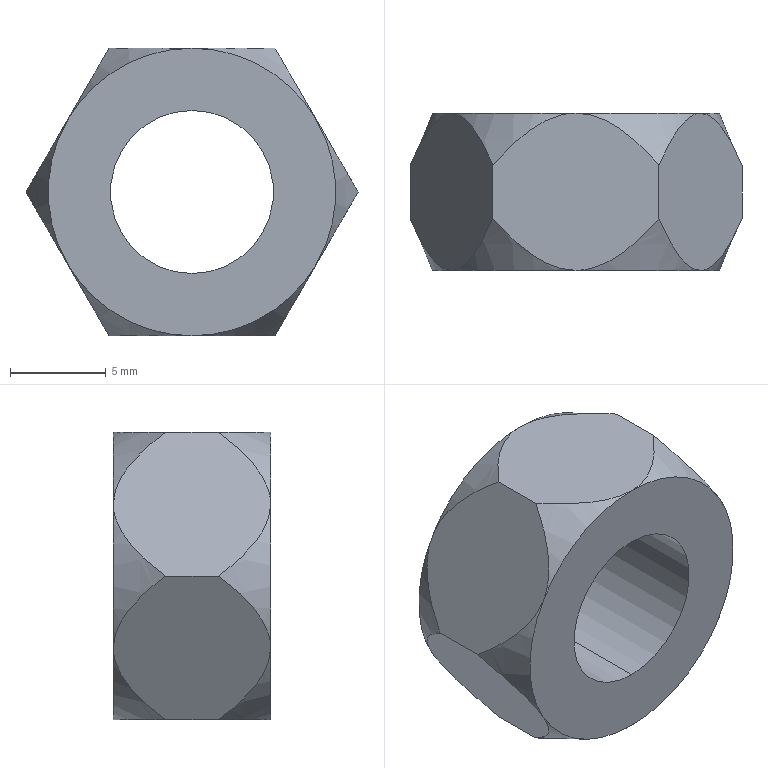Part | SolidWorks | features ICE 2, Extrusion 1, HoleWzd 1 | 1 solid | 24 faces | box 17.321 x 8.2 x 15 mm | volume 1094 mm3 | cone 14 | plane 8 | cylinder 2 | commonest cylinder face diameters 8.5 x2
STEP:
#1=CARTESIAN_POINT('',(0.,7.425,-4.25));
#2=VERTEX_POINT('',#1);
#3=CARTESIAN_POINT('',(0.,7.425,4.25));
#4=VERTEX_POINT('',#3);
#5=CARTESIAN_POINT('',(0.,7.425,0.));
#6=DIRECTION('',(0.,1.,0.));
#7=DIRECTION('',(0.,0.,1.));
#8=AXIS2_PLACEMENT_3D('',#5,#6,#7);
#9=CIRCLE('',#8,4.25);
#10=EDGE_CURVE('',#2,#4,#9,.T.);
#11=ORIENTED_EDGE('',*,*,#10,.F.);
#12=CARTESIAN_POINT('',(0.,8.2,-5.025));
#13=VERTEX_POINT('',#12);
#14=CARTESIAN_POINT('',(0.,8.2,-5.025));
#15=DIRECTION('',(0.,0.7071,-0.7071));
#16=VECTOR('',#15,1000.);
#17=LINE('',#14,#16);
#18=EDGE_CURVE('',#2,#13,#17,.T.);
#19=ORIENTED_EDGE('',*,*,#18,.T.);
#20=CARTESIAN_POINT('',(0.,8.2,5.025));
#21=VERTEX_POINT('',#20);
#22=CARTESIAN_POINT('',(0.,8.2,0.));
#23=DIRECTION('',(0.,1.,0.));
#24=DIRECTION('',(0.,0.,1.));
#25=AXIS2_PLACEMENT_3D('',#22,#23,#24);
#26=CIRCLE('',#25,5.025);
#27=EDGE_CURVE('',#13,#21,#26,.T.);
#28=ORIENTED_EDGE('',*,*,#27,.T.);
#29=CARTESIAN_POINT('',(0.,8.2,5.025));
#30=DIRECTION('',(0.,0.7071,0.7071));
#31=VECTOR('',#30,1000.);
#32=LINE('',#29,#31);
#33=EDGE_CURVE('',#4,#21,#32,.T.);
#34=ORIENTED_EDGE('',*,*,#33,.F.);
#35=EDGE_LOOP('',(#11,#19,#28,#34));
#36=FACE_OUTER_BOUND('',#35,.T.);
#37=CARTESIAN_POINT('',(0.,8.2,0.));
#38=DIRECTION('',(0.,1.,0.));
#39=DIRECTION('',(0.,0.,1.));
#40=AXIS2_PLACEMENT_3D('',#37,#38,#39);
#41=CONICAL_SURFACE('',#40,5.025,0.7854);
#42=ADVANCED_FACE('',(#36),#41,.F.);
#43=CARTESIAN_POINT('',(0.,0.,-4.25));
#44=VERTEX_POINT('',#43);
#45=CARTESIAN_POINT('',(0.,0.,4.25));
#46=VERTEX_POINT('',#45);
#47=CARTESIAN_POINT('',(0.,0.,0.));
#48=DIRECTION('',(0.,1.,0.));
#49=DIRECTION('',(0.,0.,1.));
#50=AXIS2_PLACEMENT_3D('',#47,#48,#49);
#51=CIRCLE('',#50,4.25);
#52=EDGE_CURVE('',#44,#46,#51,.T.);
#53=ORIENTED_EDGE('',*,*,#52,.F.);
#54=CARTESIAN_POINT('',(0.,8.2,-4.25));
#55=DIRECTION('',(0.,1.,0.));
#56=VECTOR('',#55,1000.);
#57=LINE('',#54,#56);
#58=EDGE_CURVE('',#44,#2,#57,.T.);
#59=ORIENTED_EDGE('',*,*,#58,.T.);
#60=ORIENTED_EDGE('',*,*,#10,.T.);
#61=CARTESIAN_POINT('',(0.,8.2,4.25));
#62=DIRECTION('',(0.,1.,0.));
#63=VECTOR('',#62,1000.);
#64=LINE('',#61,#63);
#65=EDGE_CURVE('',#46,#4,#64,.T.);
#66=ORIENTED_EDGE('',*,*,#65,.F.);
#67=EDGE_LOOP('',(#53,#59,#60,#66));
#68=FACE_OUTER_BOUND('',#67,.T.);
#69=CARTESIAN_POINT('',(0.,8.2,0.));
#70=DIRECTION('',(0.,1.,0.));
#71=DIRECTION('',(0.,0.,1.));
#72=AXIS2_PLACEMENT_3D('',#69,#70,#71);
#73=CYLINDRICAL_SURFACE('',#72,4.25);
#74=ADVANCED_FACE('',(#68),#73,.F.);
#75=CARTESIAN_POINT('',(4.33,2.733,-7.5));
#76=VERTEX_POINT('',#75);
#77=CARTESIAN_POINT('',(6.495,0.,-3.75));
#78=VERTEX_POINT('',#77);
#79=CARTESIAN_POINT('',(4.33,2.733,-7.5));
#80=CARTESIAN_POINT('',(4.473,2.397,-7.253));
#81=CARTESIAN_POINT('',(4.621,2.073,-6.997));
#82=CARTESIAN_POINT('',(4.933,1.46,-6.456));
#83=CARTESIAN_POINT('',(5.097,1.172,-6.172));
#84=CARTESIAN_POINT('',(5.452,0.6535,-5.557));
#85=CARTESIAN_POINT('',(5.645,0.4234,-5.223));
#86=CARTESIAN_POINT('',(5.952,0.1778,-4.69));
#87=CARTESIAN_POINT('',(6.06,0.1115,-4.504));
#88=CARTESIAN_POINT('',(6.276,0.02274,-4.129));
#89=CARTESIAN_POINT('',(6.385,0.,-3.94));
#90=CARTESIAN_POINT('',(6.495,0.,-3.75));
#91=B_SPLINE_CURVE_WITH_KNOTS('',3,(#79,#80,#81,#82,#83,#84,#85,#86,#87,#88,#89,#90),.UNSPECIFIED.,.F.,.F.,(4,2,2,2,2,4),(0.000000354,0.001312,0.002623,0.003934,0.00459,0.005245),.UNSPECIFIED.);
#92=EDGE_CURVE('',#76,#78,#91,.T.);
#93=ORIENTED_EDGE('',*,*,#92,.F.);
#94=CARTESIAN_POINT('',(4.33,5.467,-7.5));
#95=VERTEX_POINT('',#94);
#96=CARTESIAN_POINT('',(4.33,8.2,-7.5));
#97=DIRECTION('',(0.,-1.,0.));
#98=VECTOR('',#97,1000.);
#99=LINE('',#96,#98);
#100=EDGE_CURVE('',#95,#76,#99,.T.);
#101=ORIENTED_EDGE('',*,*,#100,.F.);
#102=CARTESIAN_POINT('',(6.495,8.2,-3.75));
#103=VERTEX_POINT('',#102);
#104=CARTESIAN_POINT('',(6.495,8.2,-3.75));
#105=CARTESIAN_POINT('',(6.386,8.2,-3.939));
#106=CARTESIAN_POINT('',(6.275,8.177,-4.132));
#107=CARTESIAN_POINT('',(6.059,8.088,-4.506));
#108=CARTESIAN_POINT('',(5.954,8.023,-4.688));
#109=CARTESIAN_POINT('',(5.749,7.86,-5.043));
#110=CARTESIAN_POINT('',(5.649,7.761,-5.216));
#111=CARTESIAN_POINT('',(5.459,7.543,-5.545));
#112=CARTESIAN_POINT('',(5.367,7.422,-5.704));
#113=CARTESIAN_POINT('',(5.102,7.036,-6.164));
#114=CARTESIAN_POINT('',(4.935,6.744,-6.452));
#115=CARTESIAN_POINT('',(4.621,6.128,-6.996));
#116=CARTESIAN_POINT('',(4.473,5.803,-7.253));
#117=CARTESIAN_POINT('',(4.33,5.467,-7.5));
#118=B_SPLINE_CURVE_WITH_KNOTS('',3,(#104,#105,#106,#107,#108,#109,#110,#111,#112,#113,#114,#115,#116,#117),.UNSPECIFIED.,.F.,.F.,(4,2,2,2,2,2,4),(0.005245,0.005897,0.00655,0.007202,0.007854,0.009159,0.01046),.UNSPECIFIED.);
#119=EDGE_CURVE('',#103,#95,#118,.T.);
#120=ORIENTED_EDGE('',*,*,#119,.F.);
#121=CARTESIAN_POINT('',(8.66,5.467,0.));
#122=VERTEX_POINT('',#121);
#123=CARTESIAN_POINT('',(8.66,5.467,0.));
#124=CARTESIAN_POINT('',(8.518,5.803,-0.247));
#125=CARTESIAN_POINT('',(8.37,6.127,-0.5033));
#126=CARTESIAN_POINT('',(8.058,6.74,-1.044));
#127=CARTESIAN_POINT('',(7.893,7.028,-1.328));
#128=CARTESIAN_POINT('',(7.538,7.546,-1.943));
#129=CARTESIAN_POINT('',(7.345,7.777,-2.277));
#130=CARTESIAN_POINT('',(7.038,8.022,-2.81));
#131=CARTESIAN_POINT('',(6.931,8.088,-2.996));
#132=CARTESIAN_POINT('',(6.714,8.177,-3.371));
#133=CARTESIAN_POINT('',(6.605,8.2,-3.56));
#134=CARTESIAN_POINT('',(6.495,8.2,-3.75));
#135=B_SPLINE_CURVE_WITH_KNOTS('',3,(#123,#124,#125,#126,#127,#128,#129,#130,#131,#132,#133,#134),.UNSPECIFIED.,.F.,.F.,(4,2,2,2,2,4),(0.000000354,0.001312,0.002623,0.003934,0.00459,0.005245),.UNSPECIFIED.);
#136=EDGE_CURVE('',#122,#103,#135,.T.);
#137=ORIENTED_EDGE('',*,*,#136,.F.);
#138=CARTESIAN_POINT('',(8.66,2.733,0.));
#139=VERTEX_POINT('',#138);
#140=CARTESIAN_POINT('',(8.66,8.2,0.));
#141=DIRECTION('',(0.,-1.,0.));
#142=VECTOR('',#141,1000.);
#143=LINE('',#140,#142);
#144=EDGE_CURVE('',#122,#139,#143,.T.);
#145=ORIENTED_EDGE('',*,*,#144,.T.);
#146=CARTESIAN_POINT('',(6.495,0.,-3.75));
#147=CARTESIAN_POINT('',(6.604,0.,-3.561));
#148=CARTESIAN_POINT('',(6.716,0.02322,-3.368));
#149=CARTESIAN_POINT('',(6.932,0.1121,-2.994));
#150=CARTESIAN_POINT('',(7.037,0.1769,-2.812));
#151=CARTESIAN_POINT('',(7.242,0.3403,-2.457));
#152=CARTESIAN_POINT('',(7.341,0.4391,-2.284));
#153=CARTESIAN_POINT('',(7.532,0.6574,-1.955));
#154=CARTESIAN_POINT('',(7.623,0.7777,-1.796));
#155=CARTESIAN_POINT('',(7.889,1.164,-1.336));
#156=CARTESIAN_POINT('',(8.055,1.456,-1.048));
#157=CARTESIAN_POINT('',(8.369,2.072,-0.504));
#158=CARTESIAN_POINT('',(8.518,2.397,-0.2471));
#159=CARTESIAN_POINT('',(8.66,2.733,0.));
#160=B_SPLINE_CURVE_WITH_KNOTS('',3,(#146,#147,#148,#149,#150,#151,#152,#153,#154,#155,#156,#157,#158,#159),.UNSPECIFIED.,.F.,.F.,(4,2,2,2,2,2,4),(0.005245,0.005897,0.00655,0.007202,0.007854,0.009159,0.01046),.UNSPECIFIED.);
#161=EDGE_CURVE('',#78,#139,#160,.T.);
#162=ORIENTED_EDGE('',*,*,#161,.F.);
#163=EDGE_LOOP('',(#93,#101,#120,#137,#145,#162));
#164=FACE_OUTER_BOUND('',#163,.T.);
#165=CARTESIAN_POINT('',(8.66,8.2,0.));
#166=DIRECTION('',(-0.866,0.,0.5));
#167=DIRECTION('',(0.5,0.,0.866));
#168=AXIS2_PLACEMENT_3D('',#165,#166,#167);
#169=PLANE('',#168);
#170=ADVANCED_FACE('',(#164),#169,.F.);
#171=CARTESIAN_POINT('',(-4.33,2.733,-7.5));
#172=VERTEX_POINT('',#171);
#173=CARTESIAN_POINT('',(0.,0.,-7.5));
#174=VERTEX_POINT('',#173);
#175=CARTESIAN_POINT('',(-4.33,2.733,-7.5));
#176=CARTESIAN_POINT('',(-4.046,2.398,-7.5));
#177=CARTESIAN_POINT('',(-3.75,2.074,-7.5));
#178=CARTESIAN_POINT('',(-3.125,1.461,-7.5));
#179=CARTESIAN_POINT('',(-2.797,1.172,-7.5));
#180=CARTESIAN_POINT('',(-2.261,0.781,-7.5));
#181=CARTESIAN_POINT('',(-2.075,0.6583,-7.5));
#182=CARTESIAN_POINT('',(-1.692,0.4386,-7.5));
#183=CARTESIAN_POINT('',(-1.494,0.3408,-7.5));
#184=CARTESIAN_POINT('',(-1.082,0.1766,-7.5));
#185=CARTESIAN_POINT('',(-0.8685,0.1109,-7.5));
#186=CARTESIAN_POINT('',(-0.4388,0.02303,-7.5));
#187=CARTESIAN_POINT('',(-0.221,0.,-7.5));
#188=CARTESIAN_POINT('',(0.,0.,-7.5));
#189=B_SPLINE_CURVE_WITH_KNOTS('',3,(#175,#176,#177,#178,#179,#180,#181,#182,#183,#184,#185,#186,#187,#188),.UNSPECIFIED.,.F.,.F.,(4,2,2,2,2,2,4),(0.02003,0.02134,0.02266,0.02332,0.02398,0.02464,0.02529),.UNSPECIFIED.);
#190=EDGE_CURVE('',#172,#174,#189,.T.);
#191=ORIENTED_EDGE('',*,*,#190,.F.);
#192=CARTESIAN_POINT('',(-4.33,5.467,-7.5));
#193=VERTEX_POINT('',#192);
#194=CARTESIAN_POINT('',(-4.33,8.2,-7.5));
#195=DIRECTION('',(0.,-1.,0.));
#196=VECTOR('',#195,1000.);
#197=LINE('',#194,#196);
#198=EDGE_CURVE('',#193,#172,#197,.T.);
#199=ORIENTED_EDGE('',*,*,#198,.F.);
#200=CARTESIAN_POINT('',(0.,8.2,-7.5));
#201=VERTEX_POINT('',#200);
#202=CARTESIAN_POINT('',(0.,8.2,-7.5));
#203=CARTESIAN_POINT('',(-0.2209,8.2,-7.5));
#204=CARTESIAN_POINT('',(-0.4444,8.176,-7.5));
#205=CARTESIAN_POINT('',(-0.8758,8.087,-7.5));
#206=CARTESIAN_POINT('',(-1.087,8.022,-7.5));
#207=CARTESIAN_POINT('',(-1.707,7.774,-7.5));
#208=CARTESIAN_POINT('',(-2.084,7.548,-7.5));
#209=CARTESIAN_POINT('',(-2.618,7.159,-7.5));
#210=CARTESIAN_POINT('',(-2.791,7.02,-7.5));
#211=CARTESIAN_POINT('',(-3.125,6.731,-7.5));
#212=CARTESIAN_POINT('',(-3.286,6.581,-7.5));
#213=CARTESIAN_POINT('',(-3.754,6.121,-7.5));
#214=CARTESIAN_POINT('',(-4.048,5.799,-7.5));
#215=CARTESIAN_POINT('',(-4.33,5.467,-7.5));
#216=B_SPLINE_CURVE_WITH_KNOTS('',3,(#202,#203,#204,#205,#206,#207,#208,#209,#210,#211,#212,#213,#214,#215),.UNSPECIFIED.,.F.,.F.,(4,2,2,2,2,2,4),(0.02529,0.02595,0.02661,0.02793,0.02858,0.02924,0.03056),.UNSPECIFIED.);
#217=EDGE_CURVE('',#201,#193,#216,.T.);
#218=ORIENTED_EDGE('',*,*,#217,.F.);
#219=CARTESIAN_POINT('',(4.33,5.467,-7.5));
#220=CARTESIAN_POINT('',(4.046,5.802,-7.5));
#221=CARTESIAN_POINT('',(3.75,6.126,-7.5));
#222=CARTESIAN_POINT('',(3.125,6.739,-7.5));
#223=CARTESIAN_POINT('',(2.797,7.028,-7.5));
#224=CARTESIAN_POINT('',(2.261,7.419,-7.5));
#225=CARTESIAN_POINT('',(2.075,7.542,-7.5));
#226=CARTESIAN_POINT('',(1.692,7.761,-7.5));
#227=CARTESIAN_POINT('',(1.494,7.859,-7.5));
#228=CARTESIAN_POINT('',(1.082,8.023,-7.5));
#229=CARTESIAN_POINT('',(0.8685,8.089,-7.5));
#230=CARTESIAN_POINT('',(0.4388,8.177,-7.5));
#231=CARTESIAN_POINT('',(0.221,8.2,-7.5));
#232=CARTESIAN_POINT('',(0.,8.2,-7.5));
#233=B_SPLINE_CURVE_WITH_KNOTS('',3,(#219,#220,#221,#222,#223,#224,#225,#226,#227,#228,#229,#230,#231,#232),.UNSPECIFIED.,.F.,.F.,(4,2,2,2,2,2,4),(0.02003,0.02134,0.02266,0.02332,0.02398,0.02464,0.02529),.UNSPECIFIED.);
#234=EDGE_CURVE('',#95,#201,#233,.T.);
#235=ORIENTED_EDGE('',*,*,#234,.F.);
#236=ORIENTED_EDGE('',*,*,#100,.T.);
#237=CARTESIAN_POINT('',(0.,0.,-7.5));
#238=CARTESIAN_POINT('',(0.2209,0.,-7.5));
#239=CARTESIAN_POINT('',(0.4444,0.02374,-7.5));
#240=CARTESIAN_POINT('',(0.8758,0.1129,-7.5));
#241=CARTESIAN_POINT('',(1.087,0.178,-7.5));
#242=CARTESIAN_POINT('',(1.707,0.4264,-7.5));
#243=CARTESIAN_POINT('',(2.084,0.6522,-7.5));
#244=CARTESIAN_POINT('',(2.618,1.041,-7.5));
#245=CARTESIAN_POINT('',(2.791,1.18,-7.5));
#246=CARTESIAN_POINT('',(3.125,1.469,-7.5));
#247=CARTESIAN_POINT('',(3.286,1.619,-7.5));
#248=CARTESIAN_POINT('',(3.754,2.079,-7.5));
#249=CARTESIAN_POINT('',(4.048,2.401,-7.5));
#250=CARTESIAN_POINT('',(4.33,2.733,-7.5));
#251=B_SPLINE_CURVE_WITH_KNOTS('',3,(#237,#238,#239,#240,#241,#242,#243,#244,#245,#246,#247,#248,#249,#250),.UNSPECIFIED.,.F.,.F.,(4,2,2,2,2,2,4),(0.02529,0.02595,0.02661,0.02793,0.02858,0.02924,0.03056),.UNSPECIFIED.);
#252=EDGE_CURVE('',#174,#76,#251,.T.);
#253=ORIENTED_EDGE('',*,*,#252,.F.);
#254=EDGE_LOOP('',(#191,#199,#218,#235,#236,#253));
#255=FACE_OUTER_BOUND('',#254,.T.);
#256=CARTESIAN_POINT('',(4.33,8.2,-7.5));
#257=DIRECTION('',(0.,0.,1.));
#258=DIRECTION('',(1.,0.,0.));
#259=AXIS2_PLACEMENT_3D('',#256,#257,#258);
#260=PLANE('',#259);
#261=ADVANCED_FACE('',(#255),#260,.F.);
#262=CARTESIAN_POINT('',(-8.66,2.733,0.));
#263=VERTEX_POINT('',#262);
#264=CARTESIAN_POINT('',(-6.495,0.,-3.75));
#265=VERTEX_POINT('',#264);
#266=CARTESIAN_POINT('',(-8.66,2.733,0.));
#267=CARTESIAN_POINT('',(-8.518,2.397,-0.247));
#268=CARTESIAN_POINT('',(-8.37,2.073,-0.5033));
#269=CARTESIAN_POINT('',(-8.058,1.46,-1.044));
#270=CARTESIAN_POINT('',(-7.893,1.172,-1.328));
#271=CARTESIAN_POINT('',(-7.538,0.6535,-1.943));
#272=CARTESIAN_POINT('',(-7.345,0.4234,-2.277));
#273=CARTESIAN_POINT('',(-7.038,0.1778,-2.81));
#274=CARTESIAN_POINT('',(-6.931,0.1115,-2.996));
#275=CARTESIAN_POINT('',(-6.714,0.02274,-3.371));
#276=CARTESIAN_POINT('',(-6.605,0.,-3.56));
#277=CARTESIAN_POINT('',(-6.495,0.,-3.75));
#278=B_SPLINE_CURVE_WITH_KNOTS('',3,(#266,#267,#268,#269,#270,#271,#272,#273,#274,#275,#276,#277),.UNSPECIFIED.,.F.,.F.,(4,2,2,2,2,4),(0.000000354,0.001312,0.002623,0.003934,0.00459,0.005245),.UNSPECIFIED.);
#279=EDGE_CURVE('',#263,#265,#278,.T.);
#280=ORIENTED_EDGE('',*,*,#279,.F.);
#281=CARTESIAN_POINT('',(-8.66,5.467,0.));
#282=VERTEX_POINT('',#281);
#283=CARTESIAN_POINT('',(-8.66,8.2,0.));
#284=DIRECTION('',(0.,-1.,0.));
#285=VECTOR('',#284,1000.);
#286=LINE('',#283,#285);
#287=EDGE_CURVE('',#282,#263,#286,.T.);
#288=ORIENTED_EDGE('',*,*,#287,.F.);
#289=CARTESIAN_POINT('',(-6.495,8.2,-3.75));
#290=VERTEX_POINT('',#289);
#291=CARTESIAN_POINT('',(-6.495,8.2,-3.75));
#292=CARTESIAN_POINT('',(-6.604,8.2,-3.561));
#293=CARTESIAN_POINT('',(-6.716,8.177,-3.368));
#294=CARTESIAN_POINT('',(-6.932,8.088,-2.994));
#295=CARTESIAN_POINT('',(-7.037,8.023,-2.812));
#296=CARTESIAN_POINT('',(-7.242,7.86,-2.457));
#297=CARTESIAN_POINT('',(-7.341,7.761,-2.284));
#298=CARTESIAN_POINT('',(-7.532,7.543,-1.955));
#299=CARTESIAN_POINT('',(-7.623,7.422,-1.796));
#300=CARTESIAN_POINT('',(-7.889,7.036,-1.336));
#301=CARTESIAN_POINT('',(-8.055,6.744,-1.048));
#302=CARTESIAN_POINT('',(-8.369,6.128,-0.504));
#303=CARTESIAN_POINT('',(-8.518,5.803,-0.2471));
#304=CARTESIAN_POINT('',(-8.66,5.467,0.));
#305=B_SPLINE_CURVE_WITH_KNOTS('',3,(#291,#292,#293,#294,#295,#296,#297,#298,#299,#300,#301,#302,#303,#304),.UNSPECIFIED.,.F.,.F.,(4,2,2,2,2,2,4),(0.005245,0.005897,0.00655,0.007202,0.007854,0.009159,0.01046),.UNSPECIFIED.);
#306=EDGE_CURVE('',#290,#282,#305,.T.);
#307=ORIENTED_EDGE('',*,*,#306,.F.);
#308=CARTESIAN_POINT('',(-4.33,5.467,-7.5));
#309=CARTESIAN_POINT('',(-4.473,5.803,-7.253));
#310=CARTESIAN_POINT('',(-4.621,6.127,-6.997));
#311=CARTESIAN_POINT('',(-4.933,6.74,-6.456));
#312=CARTESIAN_POINT('',(-5.097,7.028,-6.172));
#313=CARTESIAN_POINT('',(-5.452,7.546,-5.557));
#314=CARTESIAN_POINT('',(-5.645,7.777,-5.223));
#315=CARTESIAN_POINT('',(-5.952,8.022,-4.69));
#316=CARTESIAN_POINT('',(-6.06,8.088,-4.504));
#317=CARTESIAN_POINT('',(-6.276,8.177,-4.129));
#318=CARTESIAN_POINT('',(-6.385,8.2,-3.94));
#319=CARTESIAN_POINT('',(-6.495,8.2,-3.75));
#320=B_SPLINE_CURVE_WITH_KNOTS('',3,(#308,#309,#310,#311,#312,#313,#314,#315,#316,#317,#318,#319),.UNSPECIFIED.,.F.,.F.,(4,2,2,2,2,4),(0.000000354,0.001312,0.002623,0.003934,0.00459,0.005245),.UNSPECIFIED.);
#321=EDGE_CURVE('',#193,#290,#320,.T.);
#322=ORIENTED_EDGE('',*,*,#321,.F.);
#323=ORIENTED_EDGE('',*,*,#198,.T.);
#324=CARTESIAN_POINT('',(-6.495,0.,-3.75));
#325=CARTESIAN_POINT('',(-6.386,0.,-3.939));
#326=CARTESIAN_POINT('',(-6.275,0.02322,-4.132));
#327=CARTESIAN_POINT('',(-6.059,0.1121,-4.506));
#328=CARTESIAN_POINT('',(-5.954,0.1769,-4.688));
#329=CARTESIAN_POINT('',(-5.749,0.3403,-5.043));
#330=CARTESIAN_POINT('',(-5.649,0.4391,-5.216));
#331=CARTESIAN_POINT('',(-5.459,0.6574,-5.545));
#332=CARTESIAN_POINT('',(-5.367,0.7777,-5.704));
#333=CARTESIAN_POINT('',(-5.102,1.164,-6.164));
#334=CARTESIAN_POINT('',(-4.935,1.456,-6.452));
#335=CARTESIAN_POINT('',(-4.621,2.072,-6.996));
#336=CARTESIAN_POINT('',(-4.473,2.397,-7.253));
#337=CARTESIAN_POINT('',(-4.33,2.733,-7.5));
#338=B_SPLINE_CURVE_WITH_KNOTS('',3,(#324,#325,#326,#327,#328,#329,#330,#331,#332,#333,#334,#335,#336,#337),.UNSPECIFIED.,.F.,.F.,(4,2,2,2,2,2,4),(0.005245,0.005897,0.00655,0.007202,0.007854,0.009159,0.01046),.UNSPECIFIED.);
#339=EDGE_CURVE('',#265,#172,#338,.T.);
#340=ORIENTED_EDGE('',*,*,#339,.F.);
#341=EDGE_LOOP('',(#280,#288,#307,#322,#323,#340));
#342=FACE_OUTER_BOUND('',#341,.T.);
#343=CARTESIAN_POINT('',(-4.33,8.2,-7.5));
#344=DIRECTION('',(0.866,0.,0.5));
#345=DIRECTION('',(0.5,0.,-0.866));
#346=AXIS2_PLACEMENT_3D('',#343,#344,#345);
#347=PLANE('',#346);
#348=ADVANCED_FACE('',(#342),#347,.F.);
#349=CARTESIAN_POINT('',(-4.33,2.733,7.5));
#350=VERTEX_POINT('',#349);
#351=CARTESIAN_POINT('',(-6.495,0.,3.75));
#352=VERTEX_POINT('',#351);
#353=CARTESIAN_POINT('',(-4.33,2.733,7.5));
#354=CARTESIAN_POINT('',(-4.473,2.397,7.253));
#355=CARTESIAN_POINT('',(-4.621,2.073,6.997));
#356=CARTESIAN_POINT('',(-4.933,1.46,6.456));
#357=CARTESIAN_POINT('',(-5.097,1.172,6.172));
#358=CARTESIAN_POINT('',(-5.452,0.6535,5.557));
#359=CARTESIAN_POINT('',(-5.645,0.4234,5.223));
#360=CARTESIAN_POINT('',(-5.952,0.1778,4.69));
#361=CARTESIAN_POINT('',(-6.06,0.1115,4.504));
#362=CARTESIAN_POINT('',(-6.276,0.02274,4.129));
#363=CARTESIAN_POINT('',(-6.385,0.,3.94));
#364=CARTESIAN_POINT('',(-6.495,0.,3.75));
#365=B_SPLINE_CURVE_WITH_KNOTS('',3,(#353,#354,#355,#356,#357,#358,#359,#360,#361,#362,#363,#364),.UNSPECIFIED.,.F.,.F.,(4,2,2,2,2,4),(0.000000354,0.001312,0.002623,0.003934,0.00459,0.005245),.UNSPECIFIED.);
#366=EDGE_CURVE('',#350,#352,#365,.T.);
#367=ORIENTED_EDGE('',*,*,#366,.F.);
#368=CARTESIAN_POINT('',(-4.33,5.467,7.5));
#369=VERTEX_POINT('',#368);
#370=CARTESIAN_POINT('',(-4.33,8.2,7.5));
#371=DIRECTION('',(0.,-1.,0.));
#372=VECTOR('',#371,1000.);
#373=LINE('',#370,#372);
#374=EDGE_CURVE('',#369,#350,#373,.T.);
#375=ORIENTED_EDGE('',*,*,#374,.F.);
#376=CARTESIAN_POINT('',(-6.495,8.2,3.75));
#377=VERTEX_POINT('',#376);
#378=CARTESIAN_POINT('',(-6.495,8.2,3.75));
#379=CARTESIAN_POINT('',(-6.386,8.2,3.939));
#380=CARTESIAN_POINT('',(-6.275,8.177,4.132));
#381=CARTESIAN_POINT('',(-6.059,8.088,4.506));
#382=CARTESIAN_POINT('',(-5.954,8.023,4.688));
#383=CARTESIAN_POINT('',(-5.749,7.86,5.043));
#384=CARTESIAN_POINT('',(-5.649,7.761,5.216));
#385=CARTESIAN_POINT('',(-5.459,7.543,5.545));
#386=CARTESIAN_POINT('',(-5.367,7.422,5.704));
#387=CARTESIAN_POINT('',(-5.102,7.036,6.164));
#388=CARTESIAN_POINT('',(-4.935,6.744,6.452));
#389=CARTESIAN_POINT('',(-4.621,6.128,6.996));
#390=CARTESIAN_POINT('',(-4.473,5.803,7.253));
#391=CARTESIAN_POINT('',(-4.33,5.467,7.5));
#392=B_SPLINE_CURVE_WITH_KNOTS('',3,(#378,#379,#380,#381,#382,#383,#384,#385,#386,#387,#388,#389,#390,#391),.UNSPECIFIED.,.F.,.F.,(4,2,2,2,2,2,4),(0.005245,0.005897,0.00655,0.007202,0.007854,0.009159,0.01046),.UNSPECIFIED.);
#393=EDGE_CURVE('',#377,#369,#392,.T.);
#394=ORIENTED_EDGE('',*,*,#393,.F.);
#395=CARTESIAN_POINT('',(-8.66,5.467,0.));
#396=CARTESIAN_POINT('',(-8.518,5.803,0.247));
#397=CARTESIAN_POINT('',(-8.37,6.127,0.5033));
#398=CARTESIAN_POINT('',(-8.058,6.74,1.044));
#399=CARTESIAN_POINT('',(-7.893,7.028,1.328));
#400=CARTESIAN_POINT('',(-7.538,7.546,1.943));
#401=CARTESIAN_POINT('',(-7.345,7.777,2.277));
#402=CARTESIAN_POINT('',(-7.038,8.022,2.81));
#403=CARTESIAN_POINT('',(-6.931,8.088,2.996));
#404=CARTESIAN_POINT('',(-6.714,8.177,3.371));
#405=CARTESIAN_POINT('',(-6.605,8.2,3.56));
#406=CARTESIAN_POINT('',(-6.495,8.2,3.75));
#407=B_SPLINE_CURVE_WITH_KNOTS('',3,(#395,#396,#397,#398,#399,#400,#401,#402,#403,#404,#405,#406),.UNSPECIFIED.,.F.,.F.,(4,2,2,2,2,4),(0.000000354,0.001312,0.002623,0.003934,0.00459,0.005245),.UNSPECIFIED.);
#408=EDGE_CURVE('',#282,#377,#407,.T.);
#409=ORIENTED_EDGE('',*,*,#408,.F.);
#410=ORIENTED_EDGE('',*,*,#287,.T.);
#411=CARTESIAN_POINT('',(-6.495,0.,3.75));
#412=CARTESIAN_POINT('',(-6.604,0.,3.561));
#413=CARTESIAN_POINT('',(-6.716,0.02322,3.368));
#414=CARTESIAN_POINT('',(-6.932,0.1121,2.994));
#415=CARTESIAN_POINT('',(-7.037,0.1769,2.812));
#416=CARTESIAN_POINT('',(-7.242,0.3403,2.457));
#417=CARTESIAN_POINT('',(-7.341,0.4391,2.284));
#418=CARTESIAN_POINT('',(-7.532,0.6574,1.955));
#419=CARTESIAN_POINT('',(-7.623,0.7777,1.796));
#420=CARTESIAN_POINT('',(-7.889,1.164,1.336));
#421=CARTESIAN_POINT('',(-8.055,1.456,1.048));
#422=CARTESIAN_POINT('',(-8.369,2.072,0.504));
#423=CARTESIAN_POINT('',(-8.518,2.397,0.2471));
#424=CARTESIAN_POINT('',(-8.66,2.733,0.));
#425=B_SPLINE_CURVE_WITH_KNOTS('',3,(#411,#412,#413,#414,#415,#416,#417,#418,#419,#420,#421,#422,#423,#424),.UNSPECIFIED.,.F.,.F.,(4,2,2,2,2,2,4),(0.005245,0.005897,0.00655,0.007202,0.007854,0.009159,0.01046),.UNSPECIFIED.);
#426=EDGE_CURVE('',#352,#263,#425,.T.);
#427=ORIENTED_EDGE('',*,*,#426,.F.);
#428=EDGE_LOOP('',(#367,#375,#394,#409,#410,#427));
#429=FACE_OUTER_BOUND('',#428,.T.);
#430=CARTESIAN_POINT('',(-8.66,8.2,0.));
#431=DIRECTION('',(0.866,0.,-0.5));
#432=DIRECTION('',(-0.5,0.,-0.866));
#433=AXIS2_PLACEMENT_3D('',#430,#431,#432);
#434=PLANE('',#433);
#435=ADVANCED_FACE('',(#429),#434,.F.);
#436=CARTESIAN_POINT('',(4.33,2.733,7.5));
#437=VERTEX_POINT('',#436);
#438=CARTESIAN_POINT('',(0.,0.,7.5));
#439=VERTEX_POINT('',#438);
#440=CARTESIAN_POINT('',(4.33,2.733,7.5));
#441=CARTESIAN_POINT('',(4.046,2.398,7.5));
#442=CARTESIAN_POINT('',(3.75,2.074,7.5));
#443=CARTESIAN_POINT('',(3.125,1.461,7.5));
#444=CARTESIAN_POINT('',(2.797,1.172,7.5));
#445=CARTESIAN_POINT('',(2.261,0.781,7.5));
#446=CARTESIAN_POINT('',(2.075,0.6583,7.5));
#447=CARTESIAN_POINT('',(1.692,0.4386,7.5));
#448=CARTESIAN_POINT('',(1.494,0.3408,7.5));
#449=CARTESIAN_POINT('',(1.082,0.1766,7.5));
#450=CARTESIAN_POINT('',(0.8685,0.1109,7.5));
#451=CARTESIAN_POINT('',(0.4388,0.02303,7.5));
#452=CARTESIAN_POINT('',(0.221,0.,7.5));
#453=CARTESIAN_POINT('',(0.,0.,7.5));
#454=B_SPLINE_CURVE_WITH_KNOTS('',3,(#440,#441,#442,#443,#444,#445,#446,#447,#448,#449,#450,#451,#452,#453),.UNSPECIFIED.,.F.,.F.,(4,2,2,2,2,2,4),(0.02003,0.02134,0.02266,0.02332,0.02398,0.02464,0.02529),.UNSPECIFIED.);
#455=EDGE_CURVE('',#437,#439,#454,.T.);
#456=ORIENTED_EDGE('',*,*,#455,.F.);
#457=CARTESIAN_POINT('',(4.33,5.467,7.5));
#458=VERTEX_POINT('',#457);
#459=CARTESIAN_POINT('',(4.33,8.2,7.5));
#460=DIRECTION('',(0.,-1.,0.));
#461=VECTOR('',#460,1000.);
#462=LINE('',#459,#461);
#463=EDGE_CURVE('',#458,#437,#462,.T.);
#464=ORIENTED_EDGE('',*,*,#463,.F.);
#465=CARTESIAN_POINT('',(0.,8.2,7.5));
#466=VERTEX_POINT('',#465);
#467=CARTESIAN_POINT('',(0.,8.2,7.5));
#468=CARTESIAN_POINT('',(0.2209,8.2,7.5));
#469=CARTESIAN_POINT('',(0.4444,8.176,7.5));
#470=CARTESIAN_POINT('',(0.8758,8.087,7.5));
#471=CARTESIAN_POINT('',(1.087,8.022,7.5));
#472=CARTESIAN_POINT('',(1.707,7.774,7.5));
#473=CARTESIAN_POINT('',(2.084,7.548,7.5));
#474=CARTESIAN_POINT('',(2.618,7.159,7.5));
#475=CARTESIAN_POINT('',(2.791,7.02,7.5));
#476=CARTESIAN_POINT('',(3.125,6.731,7.5));
#477=CARTESIAN_POINT('',(3.286,6.581,7.5));
#478=CARTESIAN_POINT('',(3.754,6.121,7.5));
#479=CARTESIAN_POINT('',(4.048,5.799,7.5));
#480=CARTESIAN_POINT('',(4.33,5.467,7.5));
#481=B_SPLINE_CURVE_WITH_KNOTS('',3,(#467,#468,#469,#470,#471,#472,#473,#474,#475,#476,#477,#478,#479,#480),.UNSPECIFIED.,.F.,.F.,(4,2,2,2,2,2,4),(0.02529,0.02595,0.02661,0.02793,0.02858,0.02924,0.03056),.UNSPECIFIED.);
#482=EDGE_CURVE('',#466,#458,#481,.T.);
#483=ORIENTED_EDGE('',*,*,#482,.F.);
#484=CARTESIAN_POINT('',(-4.33,5.467,7.5));
#485=CARTESIAN_POINT('',(-4.046,5.802,7.5));
#486=CARTESIAN_POINT('',(-3.75,6.126,7.5));
#487=CARTESIAN_POINT('',(-3.125,6.739,7.5));
#488=CARTESIAN_POINT('',(-2.797,7.028,7.5));
#489=CARTESIAN_POINT('',(-2.261,7.419,7.5));
#490=CARTESIAN_POINT('',(-2.075,7.542,7.5));
#491=CARTESIAN_POINT('',(-1.692,7.761,7.5));
#492=CARTESIAN_POINT('',(-1.494,7.859,7.5));
#493=CARTESIAN_POINT('',(-1.082,8.023,7.5));
#494=CARTESIAN_POINT('',(-0.8685,8.089,7.5));
#495=CARTESIAN_POINT('',(-0.4388,8.177,7.5));
#496=CARTESIAN_POINT('',(-0.221,8.2,7.5));
#497=CARTESIAN_POINT('',(0.,8.2,7.5));
#498=B_SPLINE_CURVE_WITH_KNOTS('',3,(#484,#485,#486,#487,#488,#489,#490,#491,#492,#493,#494,#495,#496,#497),.UNSPECIFIED.,.F.,.F.,(4,2,2,2,2,2,4),(0.02003,0.02134,0.02266,0.02332,0.02398,0.02464,0.02529),.UNSPECIFIED.);
#499=EDGE_CURVE('',#369,#466,#498,.T.);
#500=ORIENTED_EDGE('',*,*,#499,.F.);
#501=ORIENTED_EDGE('',*,*,#374,.T.);
#502=CARTESIAN_POINT('',(0.,0.,7.5));
#503=CARTESIAN_POINT('',(-0.2209,0.,7.5));
#504=CARTESIAN_POINT('',(-0.4444,0.02374,7.5));
#505=CARTESIAN_POINT('',(-0.8758,0.1129,7.5));
#506=CARTESIAN_POINT('',(-1.087,0.178,7.5));
#507=CARTESIAN_POINT('',(-1.707,0.4264,7.5));
#508=CARTESIAN_POINT('',(-2.084,0.6522,7.5));
#509=CARTESIAN_POINT('',(-2.618,1.041,7.5));
#510=CARTESIAN_POINT('',(-2.791,1.18,7.5));
#511=CARTESIAN_POINT('',(-3.125,1.469,7.5));
#512=CARTESIAN_POINT('',(-3.286,1.619,7.5));
#513=CARTESIAN_POINT('',(-3.754,2.079,7.5));
#514=CARTESIAN_POINT('',(-4.048,2.401,7.5));
#515=CARTESIAN_POINT('',(-4.33,2.733,7.5));
#516=B_SPLINE_CURVE_WITH_KNOTS('',3,(#502,#503,#504,#505,#506,#507,#508,#509,#510,#511,#512,#513,#514,#515),.UNSPECIFIED.,.F.,.F.,(4,2,2,2,2,2,4),(0.02529,0.02595,0.02661,0.02793,0.02858,0.02924,0.03056),.UNSPECIFIED.);
#517=EDGE_CURVE('',#439,#350,#516,.T.);
#518=ORIENTED_EDGE('',*,*,#517,.F.);
#519=EDGE_LOOP('',(#456,#464,#483,#500,#501,#518));
#520=FACE_OUTER_BOUND('',#519,.T.);
#521=CARTESIAN_POINT('',(-4.33,8.2,7.5));
#522=DIRECTION('',(0.,0.,-1.));
#523=DIRECTION('',(-1.,0.,0.));
#524=AXIS2_PLACEMENT_3D('',#521,#522,#523);
#525=PLANE('',#524);
#526=ADVANCED_FACE('',(#520),#525,.F.);
#527=CARTESIAN_POINT('',(6.495,0.,3.75));
#528=VERTEX_POINT('',#527);
#529=CARTESIAN_POINT('',(8.66,2.733,0.));
#530=CARTESIAN_POINT('',(8.518,2.397,0.247));
#531=CARTESIAN_POINT('',(8.37,2.073,0.5033));
#532=CARTESIAN_POINT('',(8.058,1.46,1.044));
#533=CARTESIAN_POINT('',(7.893,1.172,1.328));
#534=CARTESIAN_POINT('',(7.538,0.6535,1.943));
#535=CARTESIAN_POINT('',(7.345,0.4234,2.277));
#536=CARTESIAN_POINT('',(7.038,0.1778,2.81));
#537=CARTESIAN_POINT('',(6.931,0.1115,2.996));
#538=CARTESIAN_POINT('',(6.714,0.02274,3.371));
#539=CARTESIAN_POINT('',(6.605,0.,3.56));
#540=CARTESIAN_POINT('',(6.495,0.,3.75));
#541=B_SPLINE_CURVE_WITH_KNOTS('',3,(#529,#530,#531,#532,#533,#534,#535,#536,#537,#538,#539,#540),.UNSPECIFIED.,.F.,.F.,(4,2,2,2,2,4),(0.000000354,0.001312,0.002623,0.003934,0.00459,0.005245),.UNSPECIFIED.);
#542=EDGE_CURVE('',#139,#528,#541,.T.);
#543=ORIENTED_EDGE('',*,*,#542,.F.);
#544=ORIENTED_EDGE('',*,*,#144,.F.);
#545=CARTESIAN_POINT('',(6.495,8.2,3.75));
#546=VERTEX_POINT('',#545);
#547=CARTESIAN_POINT('',(6.495,8.2,3.75));
#548=CARTESIAN_POINT('',(6.604,8.2,3.561));
#549=CARTESIAN_POINT('',(6.716,8.177,3.368));
#550=CARTESIAN_POINT('',(6.932,8.088,2.994));
#551=CARTESIAN_POINT('',(7.037,8.023,2.812));
#552=CARTESIAN_POINT('',(7.242,7.86,2.457));
#553=CARTESIAN_POINT('',(7.341,7.761,2.284));
#554=CARTESIAN_POINT('',(7.532,7.543,1.955));
#555=CARTESIAN_POINT('',(7.623,7.422,1.796));
#556=CARTESIAN_POINT('',(7.889,7.036,1.336));
#557=CARTESIAN_POINT('',(8.055,6.744,1.048));
#558=CARTESIAN_POINT('',(8.369,6.128,0.504));
#559=CARTESIAN_POINT('',(8.518,5.803,0.2471));
#560=CARTESIAN_POINT('',(8.66,5.467,0.));
#561=B_SPLINE_CURVE_WITH_KNOTS('',3,(#547,#548,#549,#550,#551,#552,#553,#554,#555,#556,#557,#558,#559,#560),.UNSPECIFIED.,.F.,.F.,(4,2,2,2,2,2,4),(0.005245,0.005897,0.00655,0.007202,0.007854,0.009159,0.01046),.UNSPECIFIED.);
#562=EDGE_CURVE('',#546,#122,#561,.T.);
#563=ORIENTED_EDGE('',*,*,#562,.F.);
#564=CARTESIAN_POINT('',(4.33,5.467,7.5));
#565=CARTESIAN_POINT('',(4.473,5.803,7.253));
#566=CARTESIAN_POINT('',(4.621,6.127,6.997));
#567=CARTESIAN_POINT('',(4.933,6.74,6.456));
#568=CARTESIAN_POINT('',(5.097,7.028,6.172));
#569=CARTESIAN_POINT('',(5.452,7.546,5.557));
#570=CARTESIAN_POINT('',(5.645,7.777,5.223));
#571=CARTESIAN_POINT('',(5.952,8.022,4.69));
#572=CARTESIAN_POINT('',(6.06,8.088,4.504));
#573=CARTESIAN_POINT('',(6.276,8.177,4.129));
#574=CARTESIAN_POINT('',(6.385,8.2,3.94));
#575=CARTESIAN_POINT('',(6.495,8.2,3.75));
#576=B_SPLINE_CURVE_WITH_KNOTS('',3,(#564,#565,#566,#567,#568,#569,#570,#571,#572,#573,#574,#575),.UNSPECIFIED.,.F.,.F.,(4,2,2,2,2,4),(0.000000354,0.001312,0.002623,0.003934,0.00459,0.005245),.UNSPECIFIED.);
#577=EDGE_CURVE('',#458,#546,#576,.T.);
#578=ORIENTED_EDGE('',*,*,#577,.F.);
#579=ORIENTED_EDGE('',*,*,#463,.T.);
#580=CARTESIAN_POINT('',(6.495,0.,3.75));
#581=CARTESIAN_POINT('',(6.386,0.,3.939));
#582=CARTESIAN_POINT('',(6.275,0.02322,4.132));
#583=CARTESIAN_POINT('',(6.059,0.1121,4.506));
#584=CARTESIAN_POINT('',(5.954,0.1769,4.688));
#585=CARTESIAN_POINT('',(5.749,0.3403,5.043));
#586=CARTESIAN_POINT('',(5.649,0.4391,5.216));
#587=CARTESIAN_POINT('',(5.459,0.6574,5.545));
#588=CARTESIAN_POINT('',(5.367,0.7777,5.704));
#589=CARTESIAN_POINT('',(5.102,1.164,6.164));
#590=CARTESIAN_POINT('',(4.935,1.456,6.452));
#591=CARTESIAN_POINT('',(4.621,2.072,6.996));
#592=CARTESIAN_POINT('',(4.473,2.397,7.253));
#593=CARTESIAN_POINT('',(4.33,2.733,7.5));
#594=B_SPLINE_CURVE_WITH_KNOTS('',3,(#580,#581,#582,#583,#584,#585,#586,#587,#588,#589,#590,#591,#592,#593),.UNSPECIFIED.,.F.,.F.,(4,2,2,2,2,2,4),(0.005245,0.005897,0.00655,0.007202,0.007854,0.009159,0.01046),.UNSPECIFIED.);
#595=EDGE_CURVE('',#528,#437,#594,.T.);
#596=ORIENTED_EDGE('',*,*,#595,.F.);
#597=EDGE_LOOP('',(#543,#544,#563,#578,#579,#596));
#598=FACE_OUTER_BOUND('',#597,.T.);
#599=CARTESIAN_POINT('',(4.33,8.2,7.5));
#600=DIRECTION('',(-0.866,0.,-0.5));
#601=DIRECTION('',(-0.5,0.,0.866));
#602=AXIS2_PLACEMENT_3D('',#599,#600,#601);
#603=PLANE('',#602);
#604=ADVANCED_FACE('',(#598),#603,.F.);
#605=ORIENTED_EDGE('',*,*,#393,.T.);
#606=ORIENTED_EDGE('',*,*,#499,.T.);
#607=CARTESIAN_POINT('',(0.,8.2,0.));
#608=DIRECTION('',(0.,1.,0.));
#609=DIRECTION('',(0.,0.,1.));
#610=AXIS2_PLACEMENT_3D('',#607,#608,#609);
#611=CIRCLE('',#610,7.5);
#612=EDGE_CURVE('',#377,#466,#611,.T.);
#613=ORIENTED_EDGE('',*,*,#612,.F.);
#614=EDGE_LOOP('',(#605,#606,#613));
#615=FACE_OUTER_BOUND('',#614,.T.);
#616=CARTESIAN_POINT('',(0.,8.2,0.));
#617=DIRECTION('',(0.,-1.,0.));
#618=DIRECTION('',(0.,0.,1.));
#619=AXIS2_PLACEMENT_3D('',#616,#617,#618);
#620=CONICAL_SURFACE('',#619,7.5,0.4014);
#621=ADVANCED_FACE('',(#615),#620,.T.);
#622=ORIENTED_EDGE('',*,*,#306,.T.);
#623=ORIENTED_EDGE('',*,*,#408,.T.);
#624=CARTESIAN_POINT('',(0.,8.2,0.));
#625=DIRECTION('',(0.,1.,0.));
#626=DIRECTION('',(0.,0.,1.));
#627=AXIS2_PLACEMENT_3D('',#624,#625,#626);
#628=CIRCLE('',#627,7.5);
#629=EDGE_CURVE('',#290,#377,#628,.T.);
#630=ORIENTED_EDGE('',*,*,#629,.F.);
#631=EDGE_LOOP('',(#622,#623,#630));
#632=FACE_OUTER_BOUND('',#631,.T.);
#633=CARTESIAN_POINT('',(0.,8.2,0.));
#634=DIRECTION('',(0.,-1.,0.));
#635=DIRECTION('',(0.,0.,1.));
#636=AXIS2_PLACEMENT_3D('',#633,#634,#635);
#637=CONICAL_SURFACE('',#636,7.5,0.4014);
#638=ADVANCED_FACE('',(#632),#637,.T.);
#639=ORIENTED_EDGE('',*,*,#217,.T.);
#640=ORIENTED_EDGE('',*,*,#321,.T.);
#641=CARTESIAN_POINT('',(0.,8.2,0.));
#642=DIRECTION('',(0.,1.,0.));
#643=DIRECTION('',(0.,0.,1.));
#644=AXIS2_PLACEMENT_3D('',#641,#642,#643);
#645=CIRCLE('',#644,7.5);
#646=EDGE_CURVE('',#201,#290,#645,.T.);
#647=ORIENTED_EDGE('',*,*,#646,.F.);
#648=EDGE_LOOP('',(#639,#640,#647));
#649=FACE_OUTER_BOUND('',#648,.T.);
#650=CARTESIAN_POINT('',(0.,8.2,0.));
#651=DIRECTION('',(0.,-1.,0.));
#652=DIRECTION('',(0.,0.,1.));
#653=AXIS2_PLACEMENT_3D('',#650,#651,#652);
#654=CONICAL_SURFACE('',#653,7.5,0.4014);
#655=ADVANCED_FACE('',(#649),#654,.T.);
#656=ORIENTED_EDGE('',*,*,#119,.T.);
#657=ORIENTED_EDGE('',*,*,#234,.T.);
#658=CARTESIAN_POINT('',(0.,8.2,0.));
#659=DIRECTION('',(0.,1.,0.));
#660=DIRECTION('',(0.,0.,1.));
#661=AXIS2_PLACEMENT_3D('',#658,#659,#660);
#662=CIRCLE('',#661,7.5);
#663=EDGE_CURVE('',#103,#201,#662,.T.);
#664=ORIENTED_EDGE('',*,*,#663,.F.);
#665=EDGE_LOOP('',(#656,#657,#664));
#666=FACE_OUTER_BOUND('',#665,.T.);
#667=CARTESIAN_POINT('',(0.,8.2,0.));
#668=DIRECTION('',(0.,-1.,0.));
#669=DIRECTION('',(0.,0.,1.));
#670=AXIS2_PLACEMENT_3D('',#667,#668,#669);
#671=CONICAL_SURFACE('',#670,7.5,0.4014);
#672=ADVANCED_FACE('',(#666),#671,.T.);
#673=ORIENTED_EDGE('',*,*,#136,.T.);
#674=CARTESIAN_POINT('',(0.,8.2,0.));
#675=DIRECTION('',(0.,1.,0.));
#676=DIRECTION('',(0.,0.,1.));
#677=AXIS2_PLACEMENT_3D('',#674,#675,#676);
#678=CIRCLE('',#677,7.5);
#679=EDGE_CURVE('',#546,#103,#678,.T.);
#680=ORIENTED_EDGE('',*,*,#679,.F.);
#681=ORIENTED_EDGE('',*,*,#562,.T.);
#682=EDGE_LOOP('',(#673,#680,#681));
#683=FACE_OUTER_BOUND('',#682,.T.);
#684=CARTESIAN_POINT('',(0.,8.2,0.));
#685=DIRECTION('',(0.,-1.,0.));
#686=DIRECTION('',(0.,0.,1.));
#687=AXIS2_PLACEMENT_3D('',#684,#685,#686);
#688=CONICAL_SURFACE('',#687,7.5,0.4014);
#689=ADVANCED_FACE('',(#683),#688,.T.);
#690=ORIENTED_EDGE('',*,*,#482,.T.);
#691=ORIENTED_EDGE('',*,*,#577,.T.);
#692=CARTESIAN_POINT('',(0.,8.2,0.));
#693=DIRECTION('',(0.,1.,0.));
#694=DIRECTION('',(0.,0.,1.));
#695=AXIS2_PLACEMENT_3D('',#692,#693,#694);
#696=CIRCLE('',#695,7.5);
#697=EDGE_CURVE('',#466,#546,#696,.T.);
#698=ORIENTED_EDGE('',*,*,#697,.F.);
#699=EDGE_LOOP('',(#690,#691,#698));
#700=FACE_OUTER_BOUND('',#699,.T.);
#701=CARTESIAN_POINT('',(0.,8.2,0.));
#702=DIRECTION('',(0.,-1.,0.));
#703=DIRECTION('',(0.,0.,1.));
#704=AXIS2_PLACEMENT_3D('',#701,#702,#703);
#705=CONICAL_SURFACE('',#704,7.5,0.4014);
#706=ADVANCED_FACE('',(#700),#705,.T.);
#707=CARTESIAN_POINT('',(0.,8.2,0.));
#708=DIRECTION('',(0.,1.,0.));
#709=DIRECTION('',(0.,0.,1.));
#710=AXIS2_PLACEMENT_3D('',#707,#708,#709);
#711=CIRCLE('',#710,5.025);
#712=EDGE_CURVE('',#21,#13,#711,.T.);
#713=ORIENTED_EDGE('',*,*,#712,.F.);
#714=ORIENTED_EDGE('',*,*,#27,.F.);
#715=EDGE_LOOP('',(#713,#714));
#716=FACE_BOUND('',#715,.T.);
#717=ORIENTED_EDGE('',*,*,#612,.T.);
#718=ORIENTED_EDGE('',*,*,#697,.T.);
#719=ORIENTED_EDGE('',*,*,#679,.T.);
#720=ORIENTED_EDGE('',*,*,#663,.T.);
#721=ORIENTED_EDGE('',*,*,#646,.T.);
#722=ORIENTED_EDGE('',*,*,#629,.T.);
#723=EDGE_LOOP('',(#717,#718,#719,#720,#721,#722));
#724=FACE_OUTER_BOUND('',#723,.T.);
#725=CARTESIAN_POINT('',(0.,8.2,0.));
#726=DIRECTION('',(0.,1.,0.));
#727=DIRECTION('',(0.,0.,1.));
#728=AXIS2_PLACEMENT_3D('',#725,#726,#727);
#729=PLANE('',#728);
#730=ADVANCED_FACE('',(#716,#724),#729,.T.);
#731=ORIENTED_EDGE('',*,*,#366,.T.);
#732=CARTESIAN_POINT('',(0.,0.,0.));
#733=DIRECTION('',(0.,1.,0.));
#734=DIRECTION('',(0.,0.,1.));
#735=AXIS2_PLACEMENT_3D('',#732,#733,#734);
#736=CIRCLE('',#735,7.5);
#737=EDGE_CURVE('',#352,#439,#736,.T.);
#738=ORIENTED_EDGE('',*,*,#737,.T.);
#739=ORIENTED_EDGE('',*,*,#517,.T.);
#740=EDGE_LOOP('',(#731,#738,#739));
#741=FACE_OUTER_BOUND('',#740,.T.);
#742=CARTESIAN_POINT('',(0.,0.,0.));
#743=DIRECTION('',(0.,1.,0.));
#744=DIRECTION('',(0.,0.,-1.));
#745=AXIS2_PLACEMENT_3D('',#742,#743,#744);
#746=CONICAL_SURFACE('',#745,7.5,0.4014);
#747=ADVANCED_FACE('',(#741),#746,.T.);
#748=ORIENTED_EDGE('',*,*,#279,.T.);
#749=CARTESIAN_POINT('',(0.,0.,0.));
#750=DIRECTION('',(0.,1.,0.));
#751=DIRECTION('',(0.,0.,1.));
#752=AXIS2_PLACEMENT_3D('',#749,#750,#751);
#753=CIRCLE('',#752,7.5);
#754=EDGE_CURVE('',#265,#352,#753,.T.);
#755=ORIENTED_EDGE('',*,*,#754,.T.);
#756=ORIENTED_EDGE('',*,*,#426,.T.);
#757=EDGE_LOOP('',(#748,#755,#756));
#758=FACE_OUTER_BOUND('',#757,.T.);
#759=CARTESIAN_POINT('',(0.,0.,0.));
#760=DIRECTION('',(0.,1.,0.));
#761=DIRECTION('',(0.,0.,-1.));
#762=AXIS2_PLACEMENT_3D('',#759,#760,#761);
#763=CONICAL_SURFACE('',#762,7.5,0.4014);
#764=ADVANCED_FACE('',(#758),#763,.T.);
#765=ORIENTED_EDGE('',*,*,#339,.T.);
#766=ORIENTED_EDGE('',*,*,#190,.T.);
#767=CARTESIAN_POINT('',(0.,0.,0.));
#768=DIRECTION('',(0.,1.,0.));
#769=DIRECTION('',(0.,0.,1.));
#770=AXIS2_PLACEMENT_3D('',#767,#768,#769);
#771=CIRCLE('',#770,7.5);
#772=EDGE_CURVE('',#174,#265,#771,.T.);
#773=ORIENTED_EDGE('',*,*,#772,.T.);
#774=EDGE_LOOP('',(#765,#766,#773));
#775=FACE_OUTER_BOUND('',#774,.T.);
#776=CARTESIAN_POINT('',(0.,0.,0.));
#777=DIRECTION('',(0.,1.,0.));
#778=DIRECTION('',(0.,0.,-1.));
#779=AXIS2_PLACEMENT_3D('',#776,#777,#778);
#780=CONICAL_SURFACE('',#779,7.5,0.4014);
#781=ADVANCED_FACE('',(#775),#780,.T.);
#782=ORIENTED_EDGE('',*,*,#252,.T.);
#783=ORIENTED_EDGE('',*,*,#92,.T.);
#784=CARTESIAN_POINT('',(0.,0.,0.));
#785=DIRECTION('',(0.,-1.,0.));
#786=DIRECTION('',(0.,0.,-1.));
#787=AXIS2_PLACEMENT_3D('',#784,#785,#786);
#788=CIRCLE('',#787,7.5);
#789=EDGE_CURVE('',#174,#78,#788,.T.);
#790=ORIENTED_EDGE('',*,*,#789,.F.);
#791=EDGE_LOOP('',(#782,#783,#790));
#792=FACE_OUTER_BOUND('',#791,.T.);
#793=CARTESIAN_POINT('',(0.,0.,0.));
#794=DIRECTION('',(0.,1.,0.));
#795=DIRECTION('',(0.,0.,-1.));
#796=AXIS2_PLACEMENT_3D('',#793,#794,#795);
#797=CONICAL_SURFACE('',#796,7.5,0.4014);
#798=ADVANCED_FACE('',(#792),#797,.T.);
#799=ORIENTED_EDGE('',*,*,#161,.T.);
#800=ORIENTED_EDGE('',*,*,#542,.T.);
#801=CARTESIAN_POINT('',(0.,0.,0.));
#802=DIRECTION('',(0.,1.,0.));
#803=DIRECTION('',(0.,0.,1.));
#804=AXIS2_PLACEMENT_3D('',#801,#802,#803);
#805=CIRCLE('',#804,7.5);
#806=EDGE_CURVE('',#528,#78,#805,.T.);
#807=ORIENTED_EDGE('',*,*,#806,.T.);
#808=EDGE_LOOP('',(#799,#800,#807));
#809=FACE_OUTER_BOUND('',#808,.T.);
#810=CARTESIAN_POINT('',(0.,0.,0.));
#811=DIRECTION('',(0.,1.,0.));
#812=DIRECTION('',(0.,0.,-1.));
#813=AXIS2_PLACEMENT_3D('',#810,#811,#812);
#814=CONICAL_SURFACE('',#813,7.5,0.4014);
#815=ADVANCED_FACE('',(#809),#814,.T.);
#816=ORIENTED_EDGE('',*,*,#455,.T.);
#817=CARTESIAN_POINT('',(0.,0.,0.));
#818=DIRECTION('',(0.,1.,0.));
#819=DIRECTION('',(0.,0.,1.));
#820=AXIS2_PLACEMENT_3D('',#817,#818,#819);
#821=CIRCLE('',#820,7.5);
#822=EDGE_CURVE('',#439,#528,#821,.T.);
#823=ORIENTED_EDGE('',*,*,#822,.T.);
#824=ORIENTED_EDGE('',*,*,#595,.T.);
#825=EDGE_LOOP('',(#816,#823,#824));
#826=FACE_OUTER_BOUND('',#825,.T.);
#827=CARTESIAN_POINT('',(0.,0.,0.));
#828=DIRECTION('',(0.,1.,0.));
#829=DIRECTION('',(0.,0.,-1.));
#830=AXIS2_PLACEMENT_3D('',#827,#828,#829);
#831=CONICAL_SURFACE('',#830,7.5,0.4014);
#832=ADVANCED_FACE('',(#826),#831,.T.);
#833=CARTESIAN_POINT('',(0.,0.,0.));
#834=DIRECTION('',(0.,1.,0.));
#835=DIRECTION('',(0.,0.,1.));
#836=AXIS2_PLACEMENT_3D('',#833,#834,#835);
#837=CIRCLE('',#836,4.25);
#838=EDGE_CURVE('',#46,#44,#837,.T.);
#839=ORIENTED_EDGE('',*,*,#838,.T.);
#840=ORIENTED_EDGE('',*,*,#52,.T.);
#841=EDGE_LOOP('',(#839,#840));
#842=FACE_BOUND('',#841,.T.);
#843=ORIENTED_EDGE('',*,*,#822,.F.);
#844=ORIENTED_EDGE('',*,*,#737,.F.);
#845=ORIENTED_EDGE('',*,*,#754,.F.);
#846=ORIENTED_EDGE('',*,*,#772,.F.);
#847=ORIENTED_EDGE('',*,*,#789,.T.);
#848=ORIENTED_EDGE('',*,*,#806,.F.);
#849=EDGE_LOOP('',(#843,#844,#845,#846,#847,#848));
#850=FACE_OUTER_BOUND('',#849,.T.);
#851=CARTESIAN_POINT('',(0.,0.,0.));
#852=DIRECTION('',(0.,1.,0.));
#853=DIRECTION('',(0.,0.,1.));
#854=AXIS2_PLACEMENT_3D('',#851,#852,#853);
#855=PLANE('',#854);
#856=ADVANCED_FACE('',(#842,#850),#855,.F.);
#857=ORIENTED_EDGE('',*,*,#58,.F.);
#858=ORIENTED_EDGE('',*,*,#838,.F.);
#859=ORIENTED_EDGE('',*,*,#65,.T.);
#860=CARTESIAN_POINT('',(0.,7.425,0.));
#861=DIRECTION('',(0.,1.,0.));
#862=DIRECTION('',(0.,0.,1.));
#863=AXIS2_PLACEMENT_3D('',#860,#861,#862);
#864=CIRCLE('',#863,4.25);
#865=EDGE_CURVE('',#4,#2,#864,.T.);
#866=ORIENTED_EDGE('',*,*,#865,.T.);
#867=EDGE_LOOP('',(#857,#858,#859,#866));
#868=FACE_OUTER_BOUND('',#867,.T.);
#869=CARTESIAN_POINT('',(0.,8.2,0.));
#870=DIRECTION('',(0.,1.,0.));
#871=DIRECTION('',(0.,0.,1.));
#872=AXIS2_PLACEMENT_3D('',#869,#870,#871);
#873=CYLINDRICAL_SURFACE('',#872,4.25);
#874=ADVANCED_FACE('',(#868),#873,.F.);
#875=ORIENTED_EDGE('',*,*,#18,.F.);
#876=ORIENTED_EDGE('',*,*,#865,.F.);
#877=ORIENTED_EDGE('',*,*,#33,.T.);
#878=ORIENTED_EDGE('',*,*,#712,.T.);
#879=EDGE_LOOP('',(#875,#876,#877,#878));
#880=FACE_OUTER_BOUND('',#879,.T.);
#881=CARTESIAN_POINT('',(0.,8.2,0.));
#882=DIRECTION('',(0.,1.,0.));
#883=DIRECTION('',(0.,0.,1.));
#884=AXIS2_PLACEMENT_3D('',#881,#882,#883);
#885=CONICAL_SURFACE('',#884,5.025,0.7854);
#886=ADVANCED_FACE('',(#880),#885,.F.);
#887=CLOSED_SHELL('',(#42,#74,#170,#261,#348,#435,#526,#604,#621,#638,#655,#672,#689,#706,#730,#747,#764,#781,#798,#815,#832,#856,#874,#886));
#888=MANIFOLD_SOLID_BREP('',#887);
#889=CARTESIAN_POINT('',(0.,0.,0.));
#890=DIRECTION('',(0.,0.,1.));
#891=DIRECTION('',(1.,0.,0.));
#892=AXIS2_PLACEMENT_3D('',#889,#890,#891);
#893=(LENGTH_UNIT()NAMED_UNIT(*)SI_UNIT(.MILLI.,.METRE.));
#894=UNCERTAINTY_MEASURE_WITH_UNIT(LENGTH_MEASURE(0.00001),#893,'','');
#895=(NAMED_UNIT(*)PLANE_ANGLE_UNIT()SI_UNIT($,.RADIAN.));
#896=(NAMED_UNIT(*)SI_UNIT($,.STERADIAN.)SOLID_ANGLE_UNIT());
#897=(GEOMETRIC_REPRESENTATION_CONTEXT(3)GLOBAL_UNCERTAINTY_ASSIGNED_CONTEXT((#894))GLOBAL_UNIT_ASSIGNED_CONTEXT((#893,#895,#896))REPRESENTATION_CONTEXT('',''));
#898=ADVANCED_BREP_SHAPE_REPRESENTATION('',(#888,#892),#897);